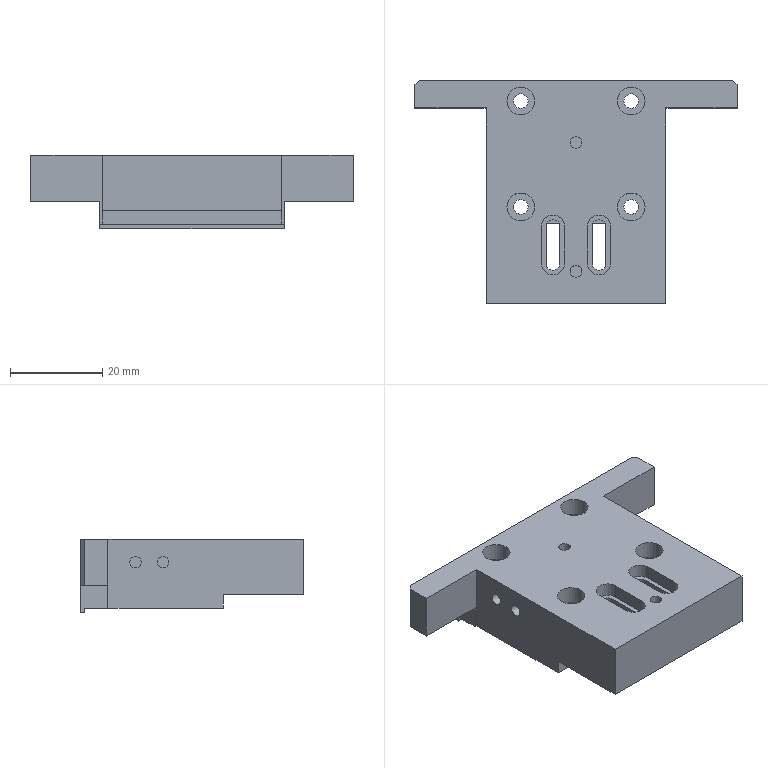NC program | NX | posted with a generic post | part box 70 x 48.5 x 16 mm
Whole program:
N10 G17 G21 G94 G90
(FLOOR_WALL_COPY , TOOL : D80)
N12 T19 M6
N14 G54
N16 G17 G0 G90 X80. Y0. S6500 M3
N18 G43 Z30. H19
N20 Z6.
N22 G94 G1 Z3. F1500.
N24 X77.
N26 X-77.
N28 X-80.
N30 Z6.
N32 G0 Z30.
N34 X80.
N36 Z5.
N38 G1 Z2.
N40 X77.
N42 X-77.
N44 X-80.
N46 Z5.
N48 G0 Z30.
N50 X80.
N52 Z4.
N54 G1 Z1.
N56 X77.
N58 X-77.
N60 X-80.
N62 Z4.
N64 G0 Z30.
N66 X80.
N68 Z3.
N70 G1 Z0.
N72 X77.
N74 X-77.
N76 X-80.
N78 Z3.
N80 G0 Z30.
N82 M5
(FLOOR_WALL_1_COPY , TOOL : D10)
N84 T15 M6
N86 G54
N88 G17 G0 G90 X-27.5 Y10.75 S9500 M3
N90 G43 Z30. H15
N92 Z2.1
N94 G94 G1 Z-0.9 F1000.
N96 X-24.5
N98 X24.5 F3000.
N100 Y9.753
N102 X-24.5
N104 Y8.757
N106 X24.5
N108 Y7.76
N110 X-24.5
N112 Y6.764
N114 X24.5
N116 Y5.767
N118 X-24.5
N120 Y4.771
N122 X24.5
N124 Y3.774
N126 X-24.5
N128 Y2.778
N130 X24.5
N132 Y1.781
N134 X-24.5
N136 Y0.784
N138 X24.5
N140 Y-0.212
N142 X-24.5
N144 Y-1.209
N146 X24.5
N148 Y-2.205
N150 X-24.5
N152 Y-3.202
N154 X24.5
N156 Y-4.198
N158 X-24.5
N160 Y-5.195
N162 X24.5
N164 Y-6.191
N166 X-24.5
N168 Y-7.188
N170 X24.5
N172 Y-8.184
N174 X-24.5
N176 Y-9.181
N178 X24.5
N180 Y-10.178
N182 X-24.5
N184 Y-11.174
N186 X24.5
N188 Y-12.171
N190 X-24.5
N192 Y-13.167
N194 X24.5
N196 X25. Y-13.25
N198 Y-14.164
N200 X-25.
N202 Y-15.16
N204 X25.
N206 Y-16.157
N208 X-25.
N210 Y-17.153
N212 X25.
N214 Y-18.15
N216 X-25.
N218 X-28.1
N220 Z2.1
N222 G0 Z30.
(FLOOR_WALL_1_COPY_COPY , TOOL : D10)
N224 X-39. Y-30.564
N226 Z-2.9
N228 G1 Z-5.9 F1000.
N230 Y-26.321
N232 Y-13.25 F3000.
N234 X-38.007
N236 Y-27.314
N238 X-37.014 Y-28.307
N240 Y-13.25
N242 X-36.021
N244 Y-29.25
N246 X-35.029
N248 Y-13.25
N250 X-34.036
N252 Y-29.25
N254 X-33.043
N256 Y-13.25
N258 X-32.05
N260 Y-29.25
N262 X-31.057
N264 Y-13.25
N266 X-30.064
N268 Y-29.25
N270 X-29.071
N272 Y-13.25
N274 X-28.079
N276 Y-29.25
N278 X-27.086
N280 Y-13.25
N282 X-26.093
N284 Y-29.25
N286 X-25.1
N288 Y-13.25
N290 Y-10.25
N292 X-27.6 Y-10.15
N294 Z-2.9
N296 G0 Z30.
N298 X39. Y-10.25
N300 Z-2.9
N302 G1 Z-5.9 F1000.
N304 Y-13.25
N306 Y-26.321 F3000.
N308 X38.007 Y-27.314
N310 Y-13.25
N312 X37.014
N314 Y-28.307
N316 X36.071 Y-29.25
N318 X36.021
N320 Y-13.25
N322 X35.029
N324 Y-29.25
N326 X34.036
N328 Y-13.25
N330 X33.043
N332 Y-29.25
N334 X32.05
N336 Y-13.25
N338 X31.057
N340 Y-29.25
N342 X30.064
N344 Y-13.25
N346 X29.071
N348 Y-29.25
N350 X28.079
N352 Y-13.25
N354 X27.086
N356 Y-29.25
N358 X26.093
N360 Y-13.25
N362 X25.1
N364 Y-29.25
N366 Y-32.35
N368 Z-2.9
N370 G0 Z30.
N372 M5
(PLANAR_MILL_COPY_COPY_COPY_COPY_COPY_COPY , TOOL : D6A45)
N374 T01 M6
N376 G54
N378 G17 G0 G90 X-21.569 Y10.97 S9500 M3
N380 G43 Z30. H1
N382 Z-3.3
N384 G94 G1 Z-4.8 F1250.
N386 X-21.149 Y10.496
N388 G3 X-20.2 Y10.179 R1.
N390 G1 Y24.15
N392 G2 X-19.4 Y24.95 R0.8
N394 G1 X19.4
N396 G2 X20.2 Y24.15 R0.8
N398 G1 Y10.179
N400 G3 X21.149 Y10.496 R1.
N402 G1 X21.569 Y10.97
N404 Z-3.3
N406 G0 Z30.
N408 X5.736 Y15.831
N410 Z-3.3
N412 G1 X5.8 Y15.721 Z-3.334
N414 Y15.5 Z-3.393
N416 Y10.25 Z-4.8
N418 Y15.5
N420 G3 X5. Y16.3 R0.8
N422 X4.2 Y15.5 R0.8
N424 G1 Y10.25
N426 G3 X5.066 Y10.75 R1.
N428 G1 Z-3.3
N430 G0 Z30.
N432 X-4.264 Y15.831
N434 Z-3.3
N436 G1 X-4.2 Y15.721 Z-3.334
N438 Y10.25 Z-4.8
N440 Y15.5
N442 G3 X-5. Y16.3 R0.8
N444 X-5.8 Y15.5 R0.8
N446 G1 Y10.25
N448 G3 X-4.934 Y10.75 R1.
N450 G1 Z-3.3
N452 G0 Z30.
N454 M5
N456 M2